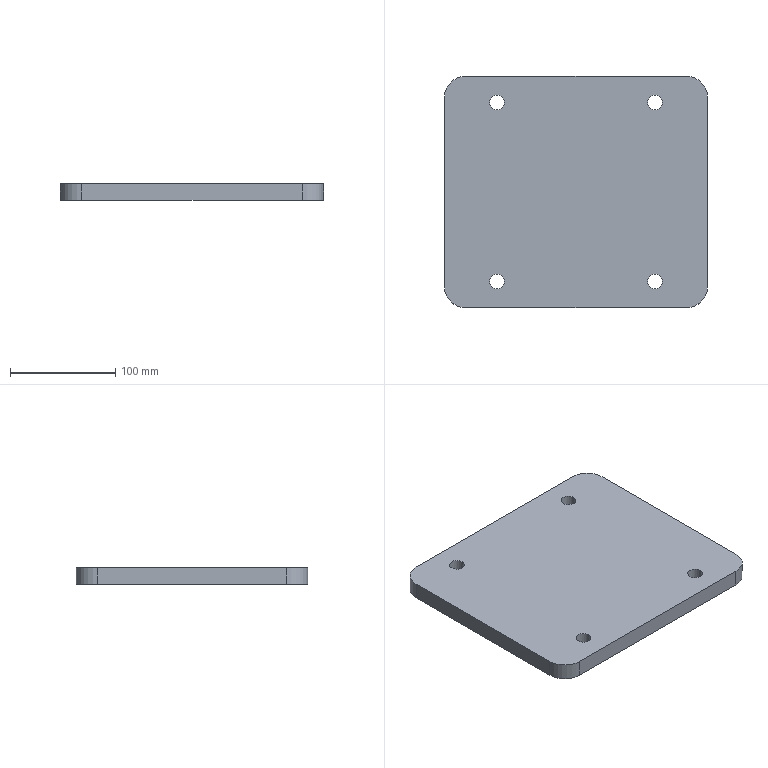Part | SolidWorks | features Chamfer 1, Extrusion 1, Fillet 1, HoleWzd 1 | 1 solid | 18 faces | box 250 x 220 x 16 mm | volume 864654 mm3 | cylinder 12 | plane 6 | commonest cylinder face diameters 14 x8 40 x4
STEP:
#1=CARTESIAN_POINT('',(-82.,85.,-8.));
#2=VERTEX_POINT('',#1);
#3=CARTESIAN_POINT('',(-68.,85.,-8.));
#4=VERTEX_POINT('',#3);
#5=CARTESIAN_POINT('',(-75.,85.,-8.));
#6=DIRECTION('',(0.,0.,1.));
#7=DIRECTION('',(1.,0.,0.));
#8=AXIS2_PLACEMENT_3D('',#5,#6,#7);
#9=CIRCLE('',#8,7.);
#10=EDGE_CURVE('',#2,#4,#9,.T.);
#11=ORIENTED_EDGE('',*,*,#10,.F.);
#12=CARTESIAN_POINT('',(-82.,85.,8.));
#13=VERTEX_POINT('',#12);
#14=CARTESIAN_POINT('',(-82.,85.,8.));
#15=DIRECTION('',(0.,0.,1.));
#16=VECTOR('',#15,1000.);
#17=LINE('',#14,#16);
#18=EDGE_CURVE('',#2,#13,#17,.T.);
#19=ORIENTED_EDGE('',*,*,#18,.T.);
#20=CARTESIAN_POINT('',(-68.,85.,8.));
#21=VERTEX_POINT('',#20);
#22=CARTESIAN_POINT('',(-75.,85.,8.));
#23=DIRECTION('',(0.,0.,1.));
#24=DIRECTION('',(1.,0.,0.));
#25=AXIS2_PLACEMENT_3D('',#22,#23,#24);
#26=CIRCLE('',#25,7.);
#27=EDGE_CURVE('',#13,#21,#26,.T.);
#28=ORIENTED_EDGE('',*,*,#27,.T.);
#29=CARTESIAN_POINT('',(-68.,85.,8.));
#30=DIRECTION('',(0.,0.,1.));
#31=VECTOR('',#30,1000.);
#32=LINE('',#29,#31);
#33=EDGE_CURVE('',#4,#21,#32,.T.);
#34=ORIENTED_EDGE('',*,*,#33,.F.);
#35=EDGE_LOOP('',(#11,#19,#28,#34));
#36=FACE_OUTER_BOUND('',#35,.T.);
#37=CARTESIAN_POINT('',(-75.,85.,8.));
#38=DIRECTION('',(0.,0.,1.));
#39=DIRECTION('',(1.,0.,0.));
#40=AXIS2_PLACEMENT_3D('',#37,#38,#39);
#41=CYLINDRICAL_SURFACE('',#40,7.);
#42=ADVANCED_FACE('',(#36),#41,.F.);
#43=CARTESIAN_POINT('',(68.,85.,-8.));
#44=VERTEX_POINT('',#43);
#45=CARTESIAN_POINT('',(82.,85.,-8.));
#46=VERTEX_POINT('',#45);
#47=CARTESIAN_POINT('',(75.,85.,-8.));
#48=DIRECTION('',(0.,0.,1.));
#49=DIRECTION('',(1.,0.,0.));
#50=AXIS2_PLACEMENT_3D('',#47,#48,#49);
#51=CIRCLE('',#50,7.);
#52=EDGE_CURVE('',#44,#46,#51,.T.);
#53=ORIENTED_EDGE('',*,*,#52,.F.);
#54=CARTESIAN_POINT('',(68.,85.,8.));
#55=VERTEX_POINT('',#54);
#56=CARTESIAN_POINT('',(68.,85.,8.));
#57=DIRECTION('',(0.,0.,1.));
#58=VECTOR('',#57,1000.);
#59=LINE('',#56,#58);
#60=EDGE_CURVE('',#44,#55,#59,.T.);
#61=ORIENTED_EDGE('',*,*,#60,.T.);
#62=CARTESIAN_POINT('',(82.,85.,8.));
#63=VERTEX_POINT('',#62);
#64=CARTESIAN_POINT('',(75.,85.,8.));
#65=DIRECTION('',(0.,0.,1.));
#66=DIRECTION('',(1.,0.,0.));
#67=AXIS2_PLACEMENT_3D('',#64,#65,#66);
#68=CIRCLE('',#67,7.);
#69=EDGE_CURVE('',#55,#63,#68,.T.);
#70=ORIENTED_EDGE('',*,*,#69,.T.);
#71=CARTESIAN_POINT('',(82.,85.,8.));
#72=DIRECTION('',(0.,0.,1.));
#73=VECTOR('',#72,1000.);
#74=LINE('',#71,#73);
#75=EDGE_CURVE('',#46,#63,#74,.T.);
#76=ORIENTED_EDGE('',*,*,#75,.F.);
#77=EDGE_LOOP('',(#53,#61,#70,#76));
#78=FACE_OUTER_BOUND('',#77,.T.);
#79=CARTESIAN_POINT('',(75.,85.,8.));
#80=DIRECTION('',(0.,0.,1.));
#81=DIRECTION('',(1.,0.,0.));
#82=AXIS2_PLACEMENT_3D('',#79,#80,#81);
#83=CYLINDRICAL_SURFACE('',#82,7.);
#84=ADVANCED_FACE('',(#78),#83,.F.);
#85=CARTESIAN_POINT('',(68.,-85.,-8.));
#86=VERTEX_POINT('',#85);
#87=CARTESIAN_POINT('',(82.,-85.,-8.));
#88=VERTEX_POINT('',#87);
#89=CARTESIAN_POINT('',(75.,-85.,-8.));
#90=DIRECTION('',(0.,0.,1.));
#91=DIRECTION('',(1.,0.,0.));
#92=AXIS2_PLACEMENT_3D('',#89,#90,#91);
#93=CIRCLE('',#92,7.);
#94=EDGE_CURVE('',#86,#88,#93,.T.);
#95=ORIENTED_EDGE('',*,*,#94,.F.);
#96=CARTESIAN_POINT('',(68.,-85.,8.));
#97=VERTEX_POINT('',#96);
#98=CARTESIAN_POINT('',(68.,-85.,8.));
#99=DIRECTION('',(0.,0.,1.));
#100=VECTOR('',#99,1000.);
#101=LINE('',#98,#100);
#102=EDGE_CURVE('',#86,#97,#101,.T.);
#103=ORIENTED_EDGE('',*,*,#102,.T.);
#104=CARTESIAN_POINT('',(82.,-85.,8.));
#105=VERTEX_POINT('',#104);
#106=CARTESIAN_POINT('',(75.,-85.,8.));
#107=DIRECTION('',(0.,0.,1.));
#108=DIRECTION('',(1.,0.,0.));
#109=AXIS2_PLACEMENT_3D('',#106,#107,#108);
#110=CIRCLE('',#109,7.);
#111=EDGE_CURVE('',#97,#105,#110,.T.);
#112=ORIENTED_EDGE('',*,*,#111,.T.);
#113=CARTESIAN_POINT('',(82.,-85.,8.));
#114=DIRECTION('',(0.,0.,1.));
#115=VECTOR('',#114,1000.);
#116=LINE('',#113,#115);
#117=EDGE_CURVE('',#88,#105,#116,.T.);
#118=ORIENTED_EDGE('',*,*,#117,.F.);
#119=EDGE_LOOP('',(#95,#103,#112,#118));
#120=FACE_OUTER_BOUND('',#119,.T.);
#121=CARTESIAN_POINT('',(75.,-85.,8.));
#122=DIRECTION('',(0.,0.,1.));
#123=DIRECTION('',(1.,0.,0.));
#124=AXIS2_PLACEMENT_3D('',#121,#122,#123);
#125=CYLINDRICAL_SURFACE('',#124,7.);
#126=ADVANCED_FACE('',(#120),#125,.F.);
#127=CARTESIAN_POINT('',(-82.,-85.,-8.));
#128=VERTEX_POINT('',#127);
#129=CARTESIAN_POINT('',(-68.,-85.,-8.));
#130=VERTEX_POINT('',#129);
#131=CARTESIAN_POINT('',(-75.,-85.,-8.));
#132=DIRECTION('',(0.,0.,1.));
#133=DIRECTION('',(1.,0.,0.));
#134=AXIS2_PLACEMENT_3D('',#131,#132,#133);
#135=CIRCLE('',#134,7.);
#136=EDGE_CURVE('',#128,#130,#135,.T.);
#137=ORIENTED_EDGE('',*,*,#136,.F.);
#138=CARTESIAN_POINT('',(-82.,-85.,8.));
#139=VERTEX_POINT('',#138);
#140=CARTESIAN_POINT('',(-82.,-85.,8.));
#141=DIRECTION('',(0.,0.,1.));
#142=VECTOR('',#141,1000.);
#143=LINE('',#140,#142);
#144=EDGE_CURVE('',#128,#139,#143,.T.);
#145=ORIENTED_EDGE('',*,*,#144,.T.);
#146=CARTESIAN_POINT('',(-68.,-85.,8.));
#147=VERTEX_POINT('',#146);
#148=CARTESIAN_POINT('',(-75.,-85.,8.));
#149=DIRECTION('',(0.,0.,1.));
#150=DIRECTION('',(1.,0.,0.));
#151=AXIS2_PLACEMENT_3D('',#148,#149,#150);
#152=CIRCLE('',#151,7.);
#153=EDGE_CURVE('',#139,#147,#152,.T.);
#154=ORIENTED_EDGE('',*,*,#153,.T.);
#155=CARTESIAN_POINT('',(-68.,-85.,8.));
#156=DIRECTION('',(0.,0.,1.));
#157=VECTOR('',#156,1000.);
#158=LINE('',#155,#157);
#159=EDGE_CURVE('',#130,#147,#158,.T.);
#160=ORIENTED_EDGE('',*,*,#159,.F.);
#161=EDGE_LOOP('',(#137,#145,#154,#160));
#162=FACE_OUTER_BOUND('',#161,.T.);
#163=CARTESIAN_POINT('',(-75.,-85.,8.));
#164=DIRECTION('',(0.,0.,1.));
#165=DIRECTION('',(1.,0.,0.));
#166=AXIS2_PLACEMENT_3D('',#163,#164,#165);
#167=CYLINDRICAL_SURFACE('',#166,7.);
#168=ADVANCED_FACE('',(#162),#167,.F.);
#169=CARTESIAN_POINT('',(-125.,90.,-8.));
#170=VERTEX_POINT('',#169);
#171=CARTESIAN_POINT('',(-125.,-90.,-8.));
#172=VERTEX_POINT('',#171);
#173=CARTESIAN_POINT('',(-125.,-110.,-8.));
#174=DIRECTION('',(0.,-1.,0.));
#175=VECTOR('',#174,1000.);
#176=LINE('',#173,#175);
#177=EDGE_CURVE('',#170,#172,#176,.T.);
#178=ORIENTED_EDGE('',*,*,#177,.T.);
#179=CARTESIAN_POINT('',(-125.,-90.,8.));
#180=VERTEX_POINT('',#179);
#181=CARTESIAN_POINT('',(-125.,-90.,8.));
#182=DIRECTION('',(0.,0.,1.));
#183=VECTOR('',#182,1000.);
#184=LINE('',#181,#183);
#185=EDGE_CURVE('',#172,#180,#184,.T.);
#186=ORIENTED_EDGE('',*,*,#185,.T.);
#187=CARTESIAN_POINT('',(-125.,90.,8.));
#188=VERTEX_POINT('',#187);
#189=CARTESIAN_POINT('',(-125.,-110.,8.));
#190=DIRECTION('',(0.,-1.,0.));
#191=VECTOR('',#190,1000.);
#192=LINE('',#189,#191);
#193=EDGE_CURVE('',#188,#180,#192,.T.);
#194=ORIENTED_EDGE('',*,*,#193,.F.);
#195=CARTESIAN_POINT('',(-125.,90.,8.));
#196=DIRECTION('',(0.,0.,-1.));
#197=VECTOR('',#196,1000.);
#198=LINE('',#195,#197);
#199=EDGE_CURVE('',#188,#170,#198,.T.);
#200=ORIENTED_EDGE('',*,*,#199,.T.);
#201=EDGE_LOOP('',(#178,#186,#194,#200));
#202=FACE_OUTER_BOUND('',#201,.T.);
#203=CARTESIAN_POINT('',(-125.,-110.,8.));
#204=DIRECTION('',(1.,0.,0.));
#205=DIRECTION('',(0.,0.,-1.));
#206=AXIS2_PLACEMENT_3D('',#203,#204,#205);
#207=PLANE('',#206);
#208=ADVANCED_FACE('',(#202),#207,.F.);
#209=CARTESIAN_POINT('',(-105.,-110.,-8.));
#210=VERTEX_POINT('',#209);
#211=CARTESIAN_POINT('',(105.,-110.,-8.));
#212=VERTEX_POINT('',#211);
#213=CARTESIAN_POINT('',(125.,-110.,-8.));
#214=DIRECTION('',(1.,0.,0.));
#215=VECTOR('',#214,1000.);
#216=LINE('',#213,#215);
#217=EDGE_CURVE('',#210,#212,#216,.T.);
#218=ORIENTED_EDGE('',*,*,#217,.T.);
#219=CARTESIAN_POINT('',(105.,-110.,8.));
#220=VERTEX_POINT('',#219);
#221=CARTESIAN_POINT('',(105.,-110.,8.));
#222=DIRECTION('',(0.,0.,1.));
#223=VECTOR('',#222,1000.);
#224=LINE('',#221,#223);
#225=EDGE_CURVE('',#212,#220,#224,.T.);
#226=ORIENTED_EDGE('',*,*,#225,.T.);
#227=CARTESIAN_POINT('',(-105.,-110.,8.));
#228=VERTEX_POINT('',#227);
#229=CARTESIAN_POINT('',(125.,-110.,8.));
#230=DIRECTION('',(1.,0.,0.));
#231=VECTOR('',#230,1000.);
#232=LINE('',#229,#231);
#233=EDGE_CURVE('',#228,#220,#232,.T.);
#234=ORIENTED_EDGE('',*,*,#233,.F.);
#235=CARTESIAN_POINT('',(-105.,-110.,8.));
#236=DIRECTION('',(0.,0.,-1.));
#237=VECTOR('',#236,1000.);
#238=LINE('',#235,#237);
#239=EDGE_CURVE('',#228,#210,#238,.T.);
#240=ORIENTED_EDGE('',*,*,#239,.T.);
#241=EDGE_LOOP('',(#218,#226,#234,#240));
#242=FACE_OUTER_BOUND('',#241,.T.);
#243=CARTESIAN_POINT('',(125.,-110.,8.));
#244=DIRECTION('',(0.,1.,0.));
#245=DIRECTION('',(-1.,0.,0.));
#246=AXIS2_PLACEMENT_3D('',#243,#244,#245);
#247=PLANE('',#246);
#248=ADVANCED_FACE('',(#242),#247,.F.);
#249=CARTESIAN_POINT('',(125.,-90.,-8.));
#250=VERTEX_POINT('',#249);
#251=CARTESIAN_POINT('',(125.,90.,-8.));
#252=VERTEX_POINT('',#251);
#253=CARTESIAN_POINT('',(125.,-110.,-8.));
#254=DIRECTION('',(0.,1.,0.));
#255=VECTOR('',#254,1000.);
#256=LINE('',#253,#255);
#257=EDGE_CURVE('',#250,#252,#256,.T.);
#258=ORIENTED_EDGE('',*,*,#257,.T.);
#259=CARTESIAN_POINT('',(125.,90.,8.));
#260=VERTEX_POINT('',#259);
#261=CARTESIAN_POINT('',(125.,90.,8.));
#262=DIRECTION('',(0.,0.,1.));
#263=VECTOR('',#262,1000.);
#264=LINE('',#261,#263);
#265=EDGE_CURVE('',#252,#260,#264,.T.);
#266=ORIENTED_EDGE('',*,*,#265,.T.);
#267=CARTESIAN_POINT('',(125.,-90.,8.));
#268=VERTEX_POINT('',#267);
#269=CARTESIAN_POINT('',(125.,-110.,8.));
#270=DIRECTION('',(0.,1.,0.));
#271=VECTOR('',#270,1000.);
#272=LINE('',#269,#271);
#273=EDGE_CURVE('',#268,#260,#272,.T.);
#274=ORIENTED_EDGE('',*,*,#273,.F.);
#275=CARTESIAN_POINT('',(125.,-90.,8.));
#276=DIRECTION('',(0.,0.,-1.));
#277=VECTOR('',#276,1000.);
#278=LINE('',#275,#277);
#279=EDGE_CURVE('',#268,#250,#278,.T.);
#280=ORIENTED_EDGE('',*,*,#279,.T.);
#281=EDGE_LOOP('',(#258,#266,#274,#280));
#282=FACE_OUTER_BOUND('',#281,.T.);
#283=CARTESIAN_POINT('',(125.,-110.,8.));
#284=DIRECTION('',(-1.,0.,0.));
#285=DIRECTION('',(0.,0.,1.));
#286=AXIS2_PLACEMENT_3D('',#283,#284,#285);
#287=PLANE('',#286);
#288=ADVANCED_FACE('',(#282),#287,.F.);
#289=CARTESIAN_POINT('',(105.,110.,8.));
#290=VERTEX_POINT('',#289);
#291=CARTESIAN_POINT('',(-105.,110.,8.));
#292=VERTEX_POINT('',#291);
#293=CARTESIAN_POINT('',(125.,110.,8.));
#294=DIRECTION('',(-1.,0.,0.));
#295=VECTOR('',#294,1000.);
#296=LINE('',#293,#295);
#297=EDGE_CURVE('',#290,#292,#296,.T.);
#298=ORIENTED_EDGE('',*,*,#297,.F.);
#299=CARTESIAN_POINT('',(105.,110.,-8.));
#300=VERTEX_POINT('',#299);
#301=CARTESIAN_POINT('',(105.,110.,8.));
#302=DIRECTION('',(0.,0.,-1.));
#303=VECTOR('',#302,1000.);
#304=LINE('',#301,#303);
#305=EDGE_CURVE('',#290,#300,#304,.T.);
#306=ORIENTED_EDGE('',*,*,#305,.T.);
#307=CARTESIAN_POINT('',(-105.,110.,-8.));
#308=VERTEX_POINT('',#307);
#309=CARTESIAN_POINT('',(125.,110.,-8.));
#310=DIRECTION('',(-1.,0.,0.));
#311=VECTOR('',#310,1000.);
#312=LINE('',#309,#311);
#313=EDGE_CURVE('',#300,#308,#312,.T.);
#314=ORIENTED_EDGE('',*,*,#313,.T.);
#315=CARTESIAN_POINT('',(-105.,110.,8.));
#316=DIRECTION('',(0.,0.,1.));
#317=VECTOR('',#316,1000.);
#318=LINE('',#315,#317);
#319=EDGE_CURVE('',#308,#292,#318,.T.);
#320=ORIENTED_EDGE('',*,*,#319,.T.);
#321=EDGE_LOOP('',(#298,#306,#314,#320));
#322=FACE_OUTER_BOUND('',#321,.T.);
#323=CARTESIAN_POINT('',(125.,110.,8.));
#324=DIRECTION('',(0.,-1.,0.));
#325=DIRECTION('',(1.,0.,0.));
#326=AXIS2_PLACEMENT_3D('',#323,#324,#325);
#327=PLANE('',#326);
#328=ADVANCED_FACE('',(#322),#327,.F.);
#329=CARTESIAN_POINT('',(-75.,85.,8.));
#330=DIRECTION('',(0.,0.,1.));
#331=DIRECTION('',(1.,0.,0.));
#332=AXIS2_PLACEMENT_3D('',#329,#330,#331);
#333=CIRCLE('',#332,7.);
#334=EDGE_CURVE('',#21,#13,#333,.T.);
#335=ORIENTED_EDGE('',*,*,#334,.F.);
#336=ORIENTED_EDGE('',*,*,#27,.F.);
#337=EDGE_LOOP('',(#335,#336));
#338=FACE_BOUND('',#337,.T.);
#339=CARTESIAN_POINT('',(75.,85.,8.));
#340=DIRECTION('',(0.,0.,1.));
#341=DIRECTION('',(1.,0.,0.));
#342=AXIS2_PLACEMENT_3D('',#339,#340,#341);
#343=CIRCLE('',#342,7.);
#344=EDGE_CURVE('',#63,#55,#343,.T.);
#345=ORIENTED_EDGE('',*,*,#344,.F.);
#346=ORIENTED_EDGE('',*,*,#69,.F.);
#347=EDGE_LOOP('',(#345,#346));
#348=FACE_BOUND('',#347,.T.);
#349=CARTESIAN_POINT('',(75.,-85.,8.));
#350=DIRECTION('',(0.,0.,1.));
#351=DIRECTION('',(1.,0.,0.));
#352=AXIS2_PLACEMENT_3D('',#349,#350,#351);
#353=CIRCLE('',#352,7.);
#354=EDGE_CURVE('',#105,#97,#353,.T.);
#355=ORIENTED_EDGE('',*,*,#354,.F.);
#356=ORIENTED_EDGE('',*,*,#111,.F.);
#357=EDGE_LOOP('',(#355,#356));
#358=FACE_BOUND('',#357,.T.);
#359=CARTESIAN_POINT('',(-75.,-85.,8.));
#360=DIRECTION('',(0.,0.,1.));
#361=DIRECTION('',(1.,0.,0.));
#362=AXIS2_PLACEMENT_3D('',#359,#360,#361);
#363=CIRCLE('',#362,7.);
#364=EDGE_CURVE('',#147,#139,#363,.T.);
#365=ORIENTED_EDGE('',*,*,#364,.F.);
#366=ORIENTED_EDGE('',*,*,#153,.F.);
#367=EDGE_LOOP('',(#365,#366));
#368=FACE_BOUND('',#367,.T.);
#369=ORIENTED_EDGE('',*,*,#273,.T.);
#370=CARTESIAN_POINT('',(105.,90.,8.));
#371=DIRECTION('',(0.,0.,1.));
#372=DIRECTION('',(1.,0.,0.));
#373=AXIS2_PLACEMENT_3D('',#370,#371,#372);
#374=CIRCLE('',#373,20.);
#375=EDGE_CURVE('',#260,#290,#374,.T.);
#376=ORIENTED_EDGE('',*,*,#375,.T.);
#377=ORIENTED_EDGE('',*,*,#297,.T.);
#378=CARTESIAN_POINT('',(-105.,90.,8.));
#379=DIRECTION('',(0.,0.,1.));
#380=DIRECTION('',(1.,0.,0.));
#381=AXIS2_PLACEMENT_3D('',#378,#379,#380);
#382=CIRCLE('',#381,20.);
#383=EDGE_CURVE('',#292,#188,#382,.T.);
#384=ORIENTED_EDGE('',*,*,#383,.T.);
#385=ORIENTED_EDGE('',*,*,#193,.T.);
#386=CARTESIAN_POINT('',(-105.,-90.,8.));
#387=DIRECTION('',(0.,0.,1.));
#388=DIRECTION('',(1.,0.,0.));
#389=AXIS2_PLACEMENT_3D('',#386,#387,#388);
#390=CIRCLE('',#389,20.);
#391=EDGE_CURVE('',#180,#228,#390,.T.);
#392=ORIENTED_EDGE('',*,*,#391,.T.);
#393=ORIENTED_EDGE('',*,*,#233,.T.);
#394=CARTESIAN_POINT('',(105.,-90.,8.));
#395=DIRECTION('',(0.,0.,1.));
#396=DIRECTION('',(1.,0.,0.));
#397=AXIS2_PLACEMENT_3D('',#394,#395,#396);
#398=CIRCLE('',#397,20.);
#399=EDGE_CURVE('',#220,#268,#398,.T.);
#400=ORIENTED_EDGE('',*,*,#399,.T.);
#401=EDGE_LOOP('',(#369,#376,#377,#384,#385,#392,#393,#400));
#402=FACE_OUTER_BOUND('',#401,.T.);
#403=CARTESIAN_POINT('',(0.,0.,8.));
#404=DIRECTION('',(0.,0.,1.));
#405=DIRECTION('',(1.,0.,0.));
#406=AXIS2_PLACEMENT_3D('',#403,#404,#405);
#407=PLANE('',#406);
#408=ADVANCED_FACE('',(#338,#348,#358,#368,#402),#407,.T.);
#409=CARTESIAN_POINT('',(-75.,85.,-8.));
#410=DIRECTION('',(0.,0.,1.));
#411=DIRECTION('',(1.,0.,0.));
#412=AXIS2_PLACEMENT_3D('',#409,#410,#411);
#413=CIRCLE('',#412,7.);
#414=EDGE_CURVE('',#4,#2,#413,.T.);
#415=ORIENTED_EDGE('',*,*,#414,.T.);
#416=ORIENTED_EDGE('',*,*,#10,.T.);
#417=EDGE_LOOP('',(#415,#416));
#418=FACE_BOUND('',#417,.T.);
#419=CARTESIAN_POINT('',(75.,85.,-8.));
#420=DIRECTION('',(0.,0.,1.));
#421=DIRECTION('',(1.,0.,0.));
#422=AXIS2_PLACEMENT_3D('',#419,#420,#421);
#423=CIRCLE('',#422,7.);
#424=EDGE_CURVE('',#46,#44,#423,.T.);
#425=ORIENTED_EDGE('',*,*,#424,.T.);
#426=ORIENTED_EDGE('',*,*,#52,.T.);
#427=EDGE_LOOP('',(#425,#426));
#428=FACE_BOUND('',#427,.T.);
#429=CARTESIAN_POINT('',(75.,-85.,-8.));
#430=DIRECTION('',(0.,0.,1.));
#431=DIRECTION('',(1.,0.,0.));
#432=AXIS2_PLACEMENT_3D('',#429,#430,#431);
#433=CIRCLE('',#432,7.);
#434=EDGE_CURVE('',#88,#86,#433,.T.);
#435=ORIENTED_EDGE('',*,*,#434,.T.);
#436=ORIENTED_EDGE('',*,*,#94,.T.);
#437=EDGE_LOOP('',(#435,#436));
#438=FACE_BOUND('',#437,.T.);
#439=CARTESIAN_POINT('',(-75.,-85.,-8.));
#440=DIRECTION('',(0.,0.,1.));
#441=DIRECTION('',(1.,0.,0.));
#442=AXIS2_PLACEMENT_3D('',#439,#440,#441);
#443=CIRCLE('',#442,7.);
#444=EDGE_CURVE('',#130,#128,#443,.T.);
#445=ORIENTED_EDGE('',*,*,#444,.T.);
#446=ORIENTED_EDGE('',*,*,#136,.T.);
#447=EDGE_LOOP('',(#445,#446));
#448=FACE_BOUND('',#447,.T.);
#449=ORIENTED_EDGE('',*,*,#313,.F.);
#450=CARTESIAN_POINT('',(105.,90.,-8.));
#451=DIRECTION('',(0.,0.,-1.));
#452=DIRECTION('',(1.,0.,0.));
#453=AXIS2_PLACEMENT_3D('',#450,#451,#452);
#454=CIRCLE('',#453,20.);
#455=EDGE_CURVE('',#300,#252,#454,.T.);
#456=ORIENTED_EDGE('',*,*,#455,.T.);
#457=ORIENTED_EDGE('',*,*,#257,.F.);
#458=CARTESIAN_POINT('',(105.,-90.,-8.));
#459=DIRECTION('',(0.,0.,-1.));
#460=DIRECTION('',(1.,0.,0.));
#461=AXIS2_PLACEMENT_3D('',#458,#459,#460);
#462=CIRCLE('',#461,20.);
#463=EDGE_CURVE('',#250,#212,#462,.T.);
#464=ORIENTED_EDGE('',*,*,#463,.T.);
#465=ORIENTED_EDGE('',*,*,#217,.F.);
#466=CARTESIAN_POINT('',(-105.,-90.,-8.));
#467=DIRECTION('',(0.,0.,-1.));
#468=DIRECTION('',(1.,0.,0.));
#469=AXIS2_PLACEMENT_3D('',#466,#467,#468);
#470=CIRCLE('',#469,20.);
#471=EDGE_CURVE('',#210,#172,#470,.T.);
#472=ORIENTED_EDGE('',*,*,#471,.T.);
#473=ORIENTED_EDGE('',*,*,#177,.F.);
#474=CARTESIAN_POINT('',(-105.,90.,-8.));
#475=DIRECTION('',(0.,0.,-1.));
#476=DIRECTION('',(1.,0.,0.));
#477=AXIS2_PLACEMENT_3D('',#474,#475,#476);
#478=CIRCLE('',#477,20.);
#479=EDGE_CURVE('',#170,#308,#478,.T.);
#480=ORIENTED_EDGE('',*,*,#479,.T.);
#481=EDGE_LOOP('',(#449,#456,#457,#464,#465,#472,#473,#480));
#482=FACE_OUTER_BOUND('',#481,.T.);
#483=CARTESIAN_POINT('',(0.,0.,-8.));
#484=DIRECTION('',(0.,0.,1.));
#485=DIRECTION('',(1.,0.,0.));
#486=AXIS2_PLACEMENT_3D('',#483,#484,#485);
#487=PLANE('',#486);
#488=ADVANCED_FACE('',(#418,#428,#438,#448,#482),#487,.F.);
#489=ORIENTED_EDGE('',*,*,#144,.F.);
#490=ORIENTED_EDGE('',*,*,#444,.F.);
#491=ORIENTED_EDGE('',*,*,#159,.T.);
#492=ORIENTED_EDGE('',*,*,#364,.T.);
#493=EDGE_LOOP('',(#489,#490,#491,#492));
#494=FACE_OUTER_BOUND('',#493,.T.);
#495=CARTESIAN_POINT('',(-75.,-85.,8.));
#496=DIRECTION('',(0.,0.,1.));
#497=DIRECTION('',(1.,0.,0.));
#498=AXIS2_PLACEMENT_3D('',#495,#496,#497);
#499=CYLINDRICAL_SURFACE('',#498,7.);
#500=ADVANCED_FACE('',(#494),#499,.F.);
#501=ORIENTED_EDGE('',*,*,#102,.F.);
#502=ORIENTED_EDGE('',*,*,#434,.F.);
#503=ORIENTED_EDGE('',*,*,#117,.T.);
#504=ORIENTED_EDGE('',*,*,#354,.T.);
#505=EDGE_LOOP('',(#501,#502,#503,#504));
#506=FACE_OUTER_BOUND('',#505,.T.);
#507=CARTESIAN_POINT('',(75.,-85.,8.));
#508=DIRECTION('',(0.,0.,1.));
#509=DIRECTION('',(1.,0.,0.));
#510=AXIS2_PLACEMENT_3D('',#507,#508,#509);
#511=CYLINDRICAL_SURFACE('',#510,7.);
#512=ADVANCED_FACE('',(#506),#511,.F.);
#513=ORIENTED_EDGE('',*,*,#60,.F.);
#514=ORIENTED_EDGE('',*,*,#424,.F.);
#515=ORIENTED_EDGE('',*,*,#75,.T.);
#516=ORIENTED_EDGE('',*,*,#344,.T.);
#517=EDGE_LOOP('',(#513,#514,#515,#516));
#518=FACE_OUTER_BOUND('',#517,.T.);
#519=CARTESIAN_POINT('',(75.,85.,8.));
#520=DIRECTION('',(0.,0.,1.));
#521=DIRECTION('',(1.,0.,0.));
#522=AXIS2_PLACEMENT_3D('',#519,#520,#521);
#523=CYLINDRICAL_SURFACE('',#522,7.);
#524=ADVANCED_FACE('',(#518),#523,.F.);
#525=ORIENTED_EDGE('',*,*,#18,.F.);
#526=ORIENTED_EDGE('',*,*,#414,.F.);
#527=ORIENTED_EDGE('',*,*,#33,.T.);
#528=ORIENTED_EDGE('',*,*,#334,.T.);
#529=EDGE_LOOP('',(#525,#526,#527,#528));
#530=FACE_OUTER_BOUND('',#529,.T.);
#531=CARTESIAN_POINT('',(-75.,85.,8.));
#532=DIRECTION('',(0.,0.,1.));
#533=DIRECTION('',(1.,0.,0.));
#534=AXIS2_PLACEMENT_3D('',#531,#532,#533);
#535=CYLINDRICAL_SURFACE('',#534,7.);
#536=ADVANCED_FACE('',(#530),#535,.F.);
#537=ORIENTED_EDGE('',*,*,#375,.F.);
#538=ORIENTED_EDGE('',*,*,#265,.F.);
#539=ORIENTED_EDGE('',*,*,#455,.F.);
#540=ORIENTED_EDGE('',*,*,#305,.F.);
#541=EDGE_LOOP('',(#537,#538,#539,#540));
#542=FACE_OUTER_BOUND('',#541,.T.);
#543=CARTESIAN_POINT('',(105.,90.,8.));
#544=DIRECTION('',(0.,0.,-1.));
#545=DIRECTION('',(-1.,0.,0.));
#546=AXIS2_PLACEMENT_3D('',#543,#544,#545);
#547=CYLINDRICAL_SURFACE('',#546,20.);
#548=ADVANCED_FACE('',(#542),#547,.T.);
#549=ORIENTED_EDGE('',*,*,#399,.F.);
#550=ORIENTED_EDGE('',*,*,#225,.F.);
#551=ORIENTED_EDGE('',*,*,#463,.F.);
#552=ORIENTED_EDGE('',*,*,#279,.F.);
#553=EDGE_LOOP('',(#549,#550,#551,#552));
#554=FACE_OUTER_BOUND('',#553,.T.);
#555=CARTESIAN_POINT('',(105.,-90.,8.));
#556=DIRECTION('',(0.,0.,-1.));
#557=DIRECTION('',(-1.,0.,0.));
#558=AXIS2_PLACEMENT_3D('',#555,#556,#557);
#559=CYLINDRICAL_SURFACE('',#558,20.);
#560=ADVANCED_FACE('',(#554),#559,.T.);
#561=ORIENTED_EDGE('',*,*,#391,.F.);
#562=ORIENTED_EDGE('',*,*,#185,.F.);
#563=ORIENTED_EDGE('',*,*,#471,.F.);
#564=ORIENTED_EDGE('',*,*,#239,.F.);
#565=EDGE_LOOP('',(#561,#562,#563,#564));
#566=FACE_OUTER_BOUND('',#565,.T.);
#567=CARTESIAN_POINT('',(-105.,-90.,8.));
#568=DIRECTION('',(0.,0.,-1.));
#569=DIRECTION('',(-1.,0.,0.));
#570=AXIS2_PLACEMENT_3D('',#567,#568,#569);
#571=CYLINDRICAL_SURFACE('',#570,20.);
#572=ADVANCED_FACE('',(#566),#571,.T.);
#573=ORIENTED_EDGE('',*,*,#383,.F.);
#574=ORIENTED_EDGE('',*,*,#319,.F.);
#575=ORIENTED_EDGE('',*,*,#479,.F.);
#576=ORIENTED_EDGE('',*,*,#199,.F.);
#577=EDGE_LOOP('',(#573,#574,#575,#576));
#578=FACE_OUTER_BOUND('',#577,.T.);
#579=CARTESIAN_POINT('',(-105.,90.,8.));
#580=DIRECTION('',(0.,0.,-1.));
#581=DIRECTION('',(-1.,0.,0.));
#582=AXIS2_PLACEMENT_3D('',#579,#580,#581);
#583=CYLINDRICAL_SURFACE('',#582,20.);
#584=ADVANCED_FACE('',(#578),#583,.T.);
#585=CLOSED_SHELL('',(#42,#84,#126,#168,#208,#248,#288,#328,#408,#488,#500,#512,#524,#536,#548,#560,#572,#584));
#586=MANIFOLD_SOLID_BREP('',#585);
#587=CARTESIAN_POINT('',(0.,0.,0.));
#588=DIRECTION('',(0.,0.,1.));
#589=DIRECTION('',(1.,0.,0.));
#590=AXIS2_PLACEMENT_3D('',#587,#588,#589);
#591=(LENGTH_UNIT()NAMED_UNIT(*)SI_UNIT(.MILLI.,.METRE.));
#592=UNCERTAINTY_MEASURE_WITH_UNIT(LENGTH_MEASURE(0.00001),#591,'','');
#593=(NAMED_UNIT(*)PLANE_ANGLE_UNIT()SI_UNIT($,.RADIAN.));
#594=(NAMED_UNIT(*)SI_UNIT($,.STERADIAN.)SOLID_ANGLE_UNIT());
#595=(GEOMETRIC_REPRESENTATION_CONTEXT(3)GLOBAL_UNCERTAINTY_ASSIGNED_CONTEXT((#592))GLOBAL_UNIT_ASSIGNED_CONTEXT((#591,#593,#594))REPRESENTATION_CONTEXT('',''));
#596=ADVANCED_BREP_SHAPE_REPRESENTATION('',(#586,#590),#595);